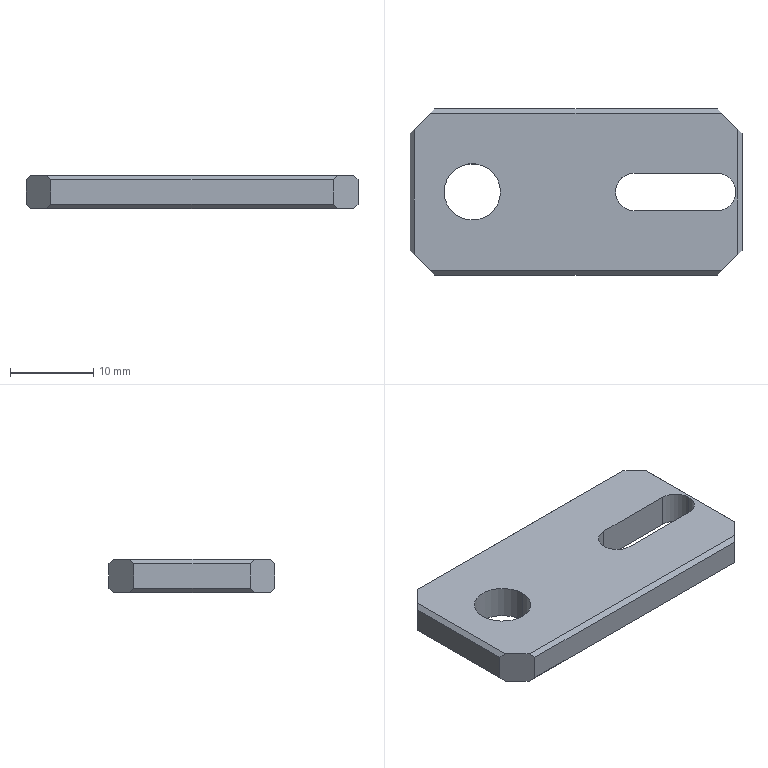Part | SolidWorks | features Chamfer 2, Extrusion 1, HoleWzd 1, ICE 1 | 1 solid | 25 faces | box 40 x 20 x 4 mm | volume 2715 mm3 | plane 20 | cylinder 5 | commonest cylinder face diameters 4.5 x3 6.8 x2
STEP:
#1=CARTESIAN_POINT('',(19.25,0.,0.));
#2=VERTEX_POINT('',#1);
#3=CARTESIAN_POINT('',(17.,2.25,0.));
#4=VERTEX_POINT('',#3);
#5=CARTESIAN_POINT('',(17.,0.,0.));
#6=DIRECTION('',(0.,0.,1.));
#7=DIRECTION('',(1.,0.,0.));
#8=AXIS2_PLACEMENT_3D('',#5,#6,#7);
#9=CIRCLE('',#8,2.25);
#10=EDGE_CURVE('',#2,#4,#9,.T.);
#11=ORIENTED_EDGE('',*,*,#10,.F.);
#12=CARTESIAN_POINT('',(19.25,0.,4.));
#13=VERTEX_POINT('',#12);
#14=CARTESIAN_POINT('',(19.25,0.,0.));
#15=DIRECTION('',(0.,0.,1.));
#16=VECTOR('',#15,1000.);
#17=LINE('',#14,#16);
#18=EDGE_CURVE('',#2,#13,#17,.T.);
#19=ORIENTED_EDGE('',*,*,#18,.T.);
#20=CARTESIAN_POINT('',(17.,2.25,4.));
#21=VERTEX_POINT('',#20);
#22=CARTESIAN_POINT('',(17.,0.,4.));
#23=DIRECTION('',(0.,0.,1.));
#24=DIRECTION('',(1.,0.,0.));
#25=AXIS2_PLACEMENT_3D('',#22,#23,#24);
#26=CIRCLE('',#25,2.25);
#27=EDGE_CURVE('',#13,#21,#26,.T.);
#28=ORIENTED_EDGE('',*,*,#27,.T.);
#29=CARTESIAN_POINT('',(17.,2.25,0.));
#30=DIRECTION('',(0.,0.,1.));
#31=VECTOR('',#30,1000.);
#32=LINE('',#29,#31);
#33=EDGE_CURVE('',#4,#21,#32,.T.);
#34=ORIENTED_EDGE('',*,*,#33,.F.);
#35=EDGE_LOOP('',(#11,#19,#28,#34));
#36=FACE_OUTER_BOUND('',#35,.T.);
#37=CARTESIAN_POINT('',(17.,0.,0.));
#38=DIRECTION('',(0.,0.,1.));
#39=DIRECTION('',(1.,0.,0.));
#40=AXIS2_PLACEMENT_3D('',#37,#38,#39);
#41=CYLINDRICAL_SURFACE('',#40,2.25);
#42=ADVANCED_FACE('',(#36),#41,.F.);
#43=CARTESIAN_POINT('',(-15.9,0.,0.));
#44=VERTEX_POINT('',#43);
#45=CARTESIAN_POINT('',(-9.1,0.,0.));
#46=VERTEX_POINT('',#45);
#47=CARTESIAN_POINT('',(-12.5,0.,0.));
#48=DIRECTION('',(0.,0.,1.));
#49=DIRECTION('',(1.,0.,0.));
#50=AXIS2_PLACEMENT_3D('',#47,#48,#49);
#51=CIRCLE('',#50,3.4);
#52=EDGE_CURVE('',#44,#46,#51,.T.);
#53=ORIENTED_EDGE('',*,*,#52,.F.);
#54=CARTESIAN_POINT('',(-15.9,0.,4.));
#55=VERTEX_POINT('',#54);
#56=CARTESIAN_POINT('',(-15.9,0.,4.));
#57=DIRECTION('',(0.,0.,1.));
#58=VECTOR('',#57,1000.);
#59=LINE('',#56,#58);
#60=EDGE_CURVE('',#44,#55,#59,.T.);
#61=ORIENTED_EDGE('',*,*,#60,.T.);
#62=CARTESIAN_POINT('',(-9.1,0.,4.));
#63=VERTEX_POINT('',#62);
#64=CARTESIAN_POINT('',(-12.5,0.,4.));
#65=DIRECTION('',(0.,0.,1.));
#66=DIRECTION('',(1.,0.,0.));
#67=AXIS2_PLACEMENT_3D('',#64,#65,#66);
#68=CIRCLE('',#67,3.4);
#69=EDGE_CURVE('',#55,#63,#68,.T.);
#70=ORIENTED_EDGE('',*,*,#69,.T.);
#71=CARTESIAN_POINT('',(-9.1,0.,4.));
#72=DIRECTION('',(0.,0.,1.));
#73=VECTOR('',#72,1000.);
#74=LINE('',#71,#73);
#75=EDGE_CURVE('',#46,#63,#74,.T.);
#76=ORIENTED_EDGE('',*,*,#75,.F.);
#77=EDGE_LOOP('',(#53,#61,#70,#76));
#78=FACE_OUTER_BOUND('',#77,.T.);
#79=CARTESIAN_POINT('',(-12.5,0.,4.));
#80=DIRECTION('',(0.,0.,1.));
#81=DIRECTION('',(1.,0.,0.));
#82=AXIS2_PLACEMENT_3D('',#79,#80,#81);
#83=CYLINDRICAL_SURFACE('',#82,3.4);
#84=ADVANCED_FACE('',(#78),#83,.F.);
#85=CARTESIAN_POINT('',(20.,-7.,3.5));
#86=VERTEX_POINT('',#85);
#87=CARTESIAN_POINT('',(20.,-7.,0.5));
#88=VERTEX_POINT('',#87);
#89=CARTESIAN_POINT('',(20.,-7.,4.));
#90=DIRECTION('',(0.,0.,-1.));
#91=VECTOR('',#90,1000.);
#92=LINE('',#89,#91);
#93=EDGE_CURVE('',#86,#88,#92,.T.);
#94=ORIENTED_EDGE('',*,*,#93,.T.);
#95=CARTESIAN_POINT('',(20.,7.,0.5));
#96=VERTEX_POINT('',#95);
#97=CARTESIAN_POINT('',(20.,7.,0.5));
#98=DIRECTION('',(0.,1.,0.));
#99=VECTOR('',#98,1000.);
#100=LINE('',#97,#99);
#101=EDGE_CURVE('',#88,#96,#100,.T.);
#102=ORIENTED_EDGE('',*,*,#101,.T.);
#103=CARTESIAN_POINT('',(20.,7.,3.5));
#104=VERTEX_POINT('',#103);
#105=CARTESIAN_POINT('',(20.,7.,4.));
#106=DIRECTION('',(0.,0.,1.));
#107=VECTOR('',#106,1000.);
#108=LINE('',#105,#107);
#109=EDGE_CURVE('',#96,#104,#108,.T.);
#110=ORIENTED_EDGE('',*,*,#109,.T.);
#111=CARTESIAN_POINT('',(20.,-10.,3.5));
#112=DIRECTION('',(0.,-1.,0.));
#113=VECTOR('',#112,1000.);
#114=LINE('',#111,#113);
#115=EDGE_CURVE('',#104,#86,#114,.T.);
#116=ORIENTED_EDGE('',*,*,#115,.T.);
#117=EDGE_LOOP('',(#94,#102,#110,#116));
#118=FACE_OUTER_BOUND('',#117,.T.);
#119=CARTESIAN_POINT('',(20.,-10.,4.));
#120=DIRECTION('',(-1.,0.,0.));
#121=DIRECTION('',(0.,0.,1.));
#122=AXIS2_PLACEMENT_3D('',#119,#120,#121);
#123=PLANE('',#122);
#124=ADVANCED_FACE('',(#118),#123,.F.);
#125=CARTESIAN_POINT('',(17.,10.,3.5));
#126=VERTEX_POINT('',#125);
#127=CARTESIAN_POINT('',(17.,10.,0.5));
#128=VERTEX_POINT('',#127);
#129=CARTESIAN_POINT('',(17.,10.,4.));
#130=DIRECTION('',(0.,0.,-1.));
#131=VECTOR('',#130,1000.);
#132=LINE('',#129,#131);
#133=EDGE_CURVE('',#126,#128,#132,.T.);
#134=ORIENTED_EDGE('',*,*,#133,.T.);
#135=CARTESIAN_POINT('',(-17.,10.,0.5));
#136=VERTEX_POINT('',#135);
#137=CARTESIAN_POINT('',(-17.,10.,0.5));
#138=DIRECTION('',(-1.,0.,0.));
#139=VECTOR('',#138,1000.);
#140=LINE('',#137,#139);
#141=EDGE_CURVE('',#128,#136,#140,.T.);
#142=ORIENTED_EDGE('',*,*,#141,.T.);
#143=CARTESIAN_POINT('',(-17.,10.,3.5));
#144=VERTEX_POINT('',#143);
#145=CARTESIAN_POINT('',(-17.,10.,4.));
#146=DIRECTION('',(0.,0.,1.));
#147=VECTOR('',#146,1000.);
#148=LINE('',#145,#147);
#149=EDGE_CURVE('',#136,#144,#148,.T.);
#150=ORIENTED_EDGE('',*,*,#149,.T.);
#151=CARTESIAN_POINT('',(-20.,10.,3.5));
#152=DIRECTION('',(1.,0.,0.));
#153=VECTOR('',#152,1000.);
#154=LINE('',#151,#153);
#155=EDGE_CURVE('',#144,#126,#154,.T.);
#156=ORIENTED_EDGE('',*,*,#155,.T.);
#157=EDGE_LOOP('',(#134,#142,#150,#156));
#158=FACE_OUTER_BOUND('',#157,.T.);
#159=CARTESIAN_POINT('',(-20.,10.,4.));
#160=DIRECTION('',(0.,-1.,0.));
#161=DIRECTION('',(0.,0.,-1.));
#162=AXIS2_PLACEMENT_3D('',#159,#160,#161);
#163=PLANE('',#162);
#164=ADVANCED_FACE('',(#158),#163,.F.);
#165=CARTESIAN_POINT('',(-20.,-7.,0.5));
#166=VERTEX_POINT('',#165);
#167=CARTESIAN_POINT('',(-20.,-7.,3.5));
#168=VERTEX_POINT('',#167);
#169=CARTESIAN_POINT('',(-20.,-7.,4.));
#170=DIRECTION('',(0.,0.,1.));
#171=VECTOR('',#170,1000.);
#172=LINE('',#169,#171);
#173=EDGE_CURVE('',#166,#168,#172,.T.);
#174=ORIENTED_EDGE('',*,*,#173,.T.);
#175=CARTESIAN_POINT('',(-20.,7.,3.5));
#176=VERTEX_POINT('',#175);
#177=CARTESIAN_POINT('',(-20.,-10.,3.5));
#178=DIRECTION('',(0.,1.,0.));
#179=VECTOR('',#178,1000.);
#180=LINE('',#177,#179);
#181=EDGE_CURVE('',#168,#176,#180,.T.);
#182=ORIENTED_EDGE('',*,*,#181,.T.);
#183=CARTESIAN_POINT('',(-20.,7.,0.5));
#184=VERTEX_POINT('',#183);
#185=CARTESIAN_POINT('',(-20.,7.,4.));
#186=DIRECTION('',(0.,0.,-1.));
#187=VECTOR('',#186,1000.);
#188=LINE('',#185,#187);
#189=EDGE_CURVE('',#176,#184,#188,.T.);
#190=ORIENTED_EDGE('',*,*,#189,.T.);
#191=CARTESIAN_POINT('',(-20.,-7.,0.5));
#192=DIRECTION('',(0.,-1.,0.));
#193=VECTOR('',#192,1000.);
#194=LINE('',#191,#193);
#195=EDGE_CURVE('',#184,#166,#194,.T.);
#196=ORIENTED_EDGE('',*,*,#195,.T.);
#197=EDGE_LOOP('',(#174,#182,#190,#196));
#198=FACE_OUTER_BOUND('',#197,.T.);
#199=CARTESIAN_POINT('',(-20.,-10.,4.));
#200=DIRECTION('',(1.,0.,0.));
#201=DIRECTION('',(0.,0.,-1.));
#202=AXIS2_PLACEMENT_3D('',#199,#200,#201);
#203=PLANE('',#202);
#204=ADVANCED_FACE('',(#198),#203,.F.);
#205=CARTESIAN_POINT('',(-17.,-10.,3.5));
#206=VERTEX_POINT('',#205);
#207=CARTESIAN_POINT('',(-17.,-10.,0.5));
#208=VERTEX_POINT('',#207);
#209=CARTESIAN_POINT('',(-17.,-10.,4.));
#210=DIRECTION('',(0.,0.,-1.));
#211=VECTOR('',#210,1000.);
#212=LINE('',#209,#211);
#213=EDGE_CURVE('',#206,#208,#212,.T.);
#214=ORIENTED_EDGE('',*,*,#213,.T.);
#215=CARTESIAN_POINT('',(17.,-10.,0.5));
#216=VERTEX_POINT('',#215);
#217=CARTESIAN_POINT('',(17.,-10.,0.5));
#218=DIRECTION('',(1.,0.,0.));
#219=VECTOR('',#218,1000.);
#220=LINE('',#217,#219);
#221=EDGE_CURVE('',#208,#216,#220,.T.);
#222=ORIENTED_EDGE('',*,*,#221,.T.);
#223=CARTESIAN_POINT('',(17.,-10.,3.5));
#224=VERTEX_POINT('',#223);
#225=CARTESIAN_POINT('',(17.,-10.,4.));
#226=DIRECTION('',(0.,0.,1.));
#227=VECTOR('',#226,1000.);
#228=LINE('',#225,#227);
#229=EDGE_CURVE('',#216,#224,#228,.T.);
#230=ORIENTED_EDGE('',*,*,#229,.T.);
#231=CARTESIAN_POINT('',(-20.,-10.,3.5));
#232=DIRECTION('',(-1.,0.,0.));
#233=VECTOR('',#232,1000.);
#234=LINE('',#231,#233);
#235=EDGE_CURVE('',#224,#206,#234,.T.);
#236=ORIENTED_EDGE('',*,*,#235,.T.);
#237=EDGE_LOOP('',(#214,#222,#230,#236));
#238=FACE_OUTER_BOUND('',#237,.T.);
#239=CARTESIAN_POINT('',(-20.,-10.,4.));
#240=DIRECTION('',(0.,1.,0.));
#241=DIRECTION('',(0.,0.,1.));
#242=AXIS2_PLACEMENT_3D('',#239,#240,#241);
#243=PLANE('',#242);
#244=ADVANCED_FACE('',(#238),#243,.F.);
#245=CARTESIAN_POINT('',(7.,-2.25,4.));
#246=VERTEX_POINT('',#245);
#247=CARTESIAN_POINT('',(17.,-2.25,4.));
#248=VERTEX_POINT('',#247);
#249=CARTESIAN_POINT('',(7.,-2.25,4.));
#250=DIRECTION('',(1.,0.,0.));
#251=VECTOR('',#250,1000.);
#252=LINE('',#249,#251);
#253=EDGE_CURVE('',#246,#248,#252,.T.);
#254=ORIENTED_EDGE('',*,*,#253,.F.);
#255=CARTESIAN_POINT('',(7.,2.25,4.));
#256=VERTEX_POINT('',#255);
#257=CARTESIAN_POINT('',(7.,0.,4.));
#258=DIRECTION('',(0.,0.,1.));
#259=DIRECTION('',(1.,0.,0.));
#260=AXIS2_PLACEMENT_3D('',#257,#258,#259);
#261=CIRCLE('',#260,2.25);
#262=EDGE_CURVE('',#256,#246,#261,.T.);
#263=ORIENTED_EDGE('',*,*,#262,.F.);
#264=CARTESIAN_POINT('',(7.,2.25,4.));
#265=DIRECTION('',(-1.,0.,0.));
#266=VECTOR('',#265,1000.);
#267=LINE('',#264,#266);
#268=EDGE_CURVE('',#21,#256,#267,.T.);
#269=ORIENTED_EDGE('',*,*,#268,.F.);
#270=ORIENTED_EDGE('',*,*,#27,.F.);
#271=CARTESIAN_POINT('',(17.,0.,4.));
#272=DIRECTION('',(0.,0.,1.));
#273=DIRECTION('',(1.,0.,0.));
#274=AXIS2_PLACEMENT_3D('',#271,#272,#273);
#275=CIRCLE('',#274,2.25);
#276=EDGE_CURVE('',#248,#13,#275,.T.);
#277=ORIENTED_EDGE('',*,*,#276,.F.);
#278=EDGE_LOOP('',(#254,#263,#269,#270,#277));
#279=FACE_BOUND('',#278,.T.);
#280=CARTESIAN_POINT('',(-12.5,0.,4.));
#281=DIRECTION('',(0.,0.,1.));
#282=DIRECTION('',(1.,0.,0.));
#283=AXIS2_PLACEMENT_3D('',#280,#281,#282);
#284=CIRCLE('',#283,3.4);
#285=EDGE_CURVE('',#63,#55,#284,.T.);
#286=ORIENTED_EDGE('',*,*,#285,.F.);
#287=ORIENTED_EDGE('',*,*,#69,.F.);
#288=EDGE_LOOP('',(#286,#287));
#289=FACE_BOUND('',#288,.T.);
#290=CARTESIAN_POINT('',(17.5,-9.5,4.));
#291=VERTEX_POINT('',#290);
#292=CARTESIAN_POINT('',(19.5,-7.5,4.));
#293=VERTEX_POINT('',#292);
#294=CARTESIAN_POINT('',(20.,-7.,4.));
#295=DIRECTION('',(0.7071,0.7071,0.));
#296=VECTOR('',#295,1000.);
#297=LINE('',#294,#296);
#298=EDGE_CURVE('',#291,#293,#297,.T.);
#299=ORIENTED_EDGE('',*,*,#298,.T.);
#300=CARTESIAN_POINT('',(19.5,7.5,4.));
#301=VERTEX_POINT('',#300);
#302=CARTESIAN_POINT('',(19.5,0.,4.));
#303=DIRECTION('',(0.,1.,0.));
#304=VECTOR('',#303,1000.);
#305=LINE('',#302,#304);
#306=EDGE_CURVE('',#293,#301,#305,.T.);
#307=ORIENTED_EDGE('',*,*,#306,.T.);
#308=CARTESIAN_POINT('',(17.5,9.5,4.));
#309=VERTEX_POINT('',#308);
#310=CARTESIAN_POINT('',(17.,10.,4.));
#311=DIRECTION('',(-0.7071,0.7071,0.));
#312=VECTOR('',#311,1000.);
#313=LINE('',#310,#312);
#314=EDGE_CURVE('',#301,#309,#313,.T.);
#315=ORIENTED_EDGE('',*,*,#314,.T.);
#316=CARTESIAN_POINT('',(-17.5,9.5,4.));
#317=VERTEX_POINT('',#316);
#318=CARTESIAN_POINT('',(0.,9.5,4.));
#319=DIRECTION('',(-1.,0.,0.));
#320=VECTOR('',#319,1000.);
#321=LINE('',#318,#320);
#322=EDGE_CURVE('',#309,#317,#321,.T.);
#323=ORIENTED_EDGE('',*,*,#322,.T.);
#324=CARTESIAN_POINT('',(-19.5,7.5,4.));
#325=VERTEX_POINT('',#324);
#326=CARTESIAN_POINT('',(-20.,7.,4.));
#327=DIRECTION('',(-0.7071,-0.7071,0.));
#328=VECTOR('',#327,1000.);
#329=LINE('',#326,#328);
#330=EDGE_CURVE('',#317,#325,#329,.T.);
#331=ORIENTED_EDGE('',*,*,#330,.T.);
#332=CARTESIAN_POINT('',(-19.5,-7.5,4.));
#333=VERTEX_POINT('',#332);
#334=CARTESIAN_POINT('',(-19.5,0.,4.));
#335=DIRECTION('',(0.,-1.,0.));
#336=VECTOR('',#335,1000.);
#337=LINE('',#334,#336);
#338=EDGE_CURVE('',#325,#333,#337,.T.);
#339=ORIENTED_EDGE('',*,*,#338,.T.);
#340=CARTESIAN_POINT('',(-17.5,-9.5,4.));
#341=VERTEX_POINT('',#340);
#342=CARTESIAN_POINT('',(-17.,-10.,4.));
#343=DIRECTION('',(0.7071,-0.7071,0.));
#344=VECTOR('',#343,1000.);
#345=LINE('',#342,#344);
#346=EDGE_CURVE('',#333,#341,#345,.T.);
#347=ORIENTED_EDGE('',*,*,#346,.T.);
#348=CARTESIAN_POINT('',(0.,-9.5,4.));
#349=DIRECTION('',(1.,0.,0.));
#350=VECTOR('',#349,1000.);
#351=LINE('',#348,#350);
#352=EDGE_CURVE('',#341,#291,#351,.T.);
#353=ORIENTED_EDGE('',*,*,#352,.T.);
#354=EDGE_LOOP('',(#299,#307,#315,#323,#331,#339,#347,#353));
#355=FACE_OUTER_BOUND('',#354,.T.);
#356=CARTESIAN_POINT('',(0.,0.,4.));
#357=DIRECTION('',(0.,0.,-1.));
#358=DIRECTION('',(-1.,0.,0.));
#359=AXIS2_PLACEMENT_3D('',#356,#357,#358);
#360=PLANE('',#359);
#361=ADVANCED_FACE('',(#279,#289,#355),#360,.F.);
#362=CARTESIAN_POINT('',(7.,2.25,0.));
#363=VERTEX_POINT('',#362);
#364=CARTESIAN_POINT('',(7.,-2.25,0.));
#365=VERTEX_POINT('',#364);
#366=CARTESIAN_POINT('',(7.,0.,0.));
#367=DIRECTION('',(0.,0.,1.));
#368=DIRECTION('',(1.,0.,0.));
#369=AXIS2_PLACEMENT_3D('',#366,#367,#368);
#370=CIRCLE('',#369,2.25);
#371=EDGE_CURVE('',#363,#365,#370,.T.);
#372=ORIENTED_EDGE('',*,*,#371,.T.);
#373=CARTESIAN_POINT('',(17.,-2.25,0.));
#374=VERTEX_POINT('',#373);
#375=CARTESIAN_POINT('',(7.,-2.25,0.));
#376=DIRECTION('',(1.,0.,0.));
#377=VECTOR('',#376,1000.);
#378=LINE('',#375,#377);
#379=EDGE_CURVE('',#365,#374,#378,.T.);
#380=ORIENTED_EDGE('',*,*,#379,.T.);
#381=CARTESIAN_POINT('',(17.,0.,0.));
#382=DIRECTION('',(0.,0.,1.));
#383=DIRECTION('',(1.,0.,0.));
#384=AXIS2_PLACEMENT_3D('',#381,#382,#383);
#385=CIRCLE('',#384,2.25);
#386=EDGE_CURVE('',#374,#2,#385,.T.);
#387=ORIENTED_EDGE('',*,*,#386,.T.);
#388=ORIENTED_EDGE('',*,*,#10,.T.);
#389=CARTESIAN_POINT('',(7.,2.25,0.));
#390=DIRECTION('',(-1.,0.,0.));
#391=VECTOR('',#390,1000.);
#392=LINE('',#389,#391);
#393=EDGE_CURVE('',#4,#363,#392,.T.);
#394=ORIENTED_EDGE('',*,*,#393,.T.);
#395=EDGE_LOOP('',(#372,#380,#387,#388,#394));
#396=FACE_BOUND('',#395,.T.);
#397=CARTESIAN_POINT('',(-12.5,0.,0.));
#398=DIRECTION('',(0.,0.,1.));
#399=DIRECTION('',(1.,0.,0.));
#400=AXIS2_PLACEMENT_3D('',#397,#398,#399);
#401=CIRCLE('',#400,3.4);
#402=EDGE_CURVE('',#46,#44,#401,.T.);
#403=ORIENTED_EDGE('',*,*,#402,.T.);
#404=ORIENTED_EDGE('',*,*,#52,.T.);
#405=EDGE_LOOP('',(#403,#404));
#406=FACE_BOUND('',#405,.T.);
#407=CARTESIAN_POINT('',(17.5,9.5,0.));
#408=VERTEX_POINT('',#407);
#409=CARTESIAN_POINT('',(19.5,7.5,0.));
#410=VERTEX_POINT('',#409);
#411=CARTESIAN_POINT('',(13.5,13.5,0.));
#412=DIRECTION('',(0.7071,-0.7071,0.));
#413=VECTOR('',#412,1000.);
#414=LINE('',#411,#413);
#415=EDGE_CURVE('',#408,#410,#414,.T.);
#416=ORIENTED_EDGE('',*,*,#415,.T.);
#417=CARTESIAN_POINT('',(19.5,-7.5,0.));
#418=VERTEX_POINT('',#417);
#419=CARTESIAN_POINT('',(19.5,-7.,0.));
#420=DIRECTION('',(0.,-1.,0.));
#421=VECTOR('',#420,1000.);
#422=LINE('',#419,#421);
#423=EDGE_CURVE('',#410,#418,#422,.T.);
#424=ORIENTED_EDGE('',*,*,#423,.T.);
#425=CARTESIAN_POINT('',(17.5,-9.5,0.));
#426=VERTEX_POINT('',#425);
#427=CARTESIAN_POINT('',(13.5,-13.5,0.));
#428=DIRECTION('',(-0.7071,-0.7071,0.));
#429=VECTOR('',#428,1000.);
#430=LINE('',#427,#429);
#431=EDGE_CURVE('',#418,#426,#430,.T.);
#432=ORIENTED_EDGE('',*,*,#431,.T.);
#433=CARTESIAN_POINT('',(-17.5,-9.5,0.));
#434=VERTEX_POINT('',#433);
#435=CARTESIAN_POINT('',(-17.,-9.5,0.));
#436=DIRECTION('',(-1.,0.,0.));
#437=VECTOR('',#436,1000.);
#438=LINE('',#435,#437);
#439=EDGE_CURVE('',#426,#434,#438,.T.);
#440=ORIENTED_EDGE('',*,*,#439,.T.);
#441=CARTESIAN_POINT('',(-19.5,-7.5,0.));
#442=VERTEX_POINT('',#441);
#443=CARTESIAN_POINT('',(-13.5,-13.5,0.));
#444=DIRECTION('',(-0.7071,0.7071,0.));
#445=VECTOR('',#444,1000.);
#446=LINE('',#443,#445);
#447=EDGE_CURVE('',#434,#442,#446,.T.);
#448=ORIENTED_EDGE('',*,*,#447,.T.);
#449=CARTESIAN_POINT('',(-19.5,7.5,0.));
#450=VERTEX_POINT('',#449);
#451=CARTESIAN_POINT('',(-19.5,7.,0.));
#452=DIRECTION('',(0.,1.,0.));
#453=VECTOR('',#452,1000.);
#454=LINE('',#451,#453);
#455=EDGE_CURVE('',#442,#450,#454,.T.);
#456=ORIENTED_EDGE('',*,*,#455,.T.);
#457=CARTESIAN_POINT('',(-17.5,9.5,0.));
#458=VERTEX_POINT('',#457);
#459=CARTESIAN_POINT('',(-13.5,13.5,0.));
#460=DIRECTION('',(0.7071,0.7071,0.));
#461=VECTOR('',#460,1000.);
#462=LINE('',#459,#461);
#463=EDGE_CURVE('',#450,#458,#462,.T.);
#464=ORIENTED_EDGE('',*,*,#463,.T.);
#465=CARTESIAN_POINT('',(17.,9.5,0.));
#466=DIRECTION('',(1.,0.,0.));
#467=VECTOR('',#466,1000.);
#468=LINE('',#465,#467);
#469=EDGE_CURVE('',#458,#408,#468,.T.);
#470=ORIENTED_EDGE('',*,*,#469,.T.);
#471=EDGE_LOOP('',(#416,#424,#432,#440,#448,#456,#464,#470));
#472=FACE_OUTER_BOUND('',#471,.T.);
#473=CARTESIAN_POINT('',(0.,0.,0.));
#474=DIRECTION('',(0.,0.,-1.));
#475=DIRECTION('',(-1.,0.,0.));
#476=AXIS2_PLACEMENT_3D('',#473,#474,#475);
#477=PLANE('',#476);
#478=ADVANCED_FACE('',(#396,#406,#472),#477,.T.);
#479=ORIENTED_EDGE('',*,*,#60,.F.);
#480=ORIENTED_EDGE('',*,*,#402,.F.);
#481=ORIENTED_EDGE('',*,*,#75,.T.);
#482=ORIENTED_EDGE('',*,*,#285,.T.);
#483=EDGE_LOOP('',(#479,#480,#481,#482));
#484=FACE_OUTER_BOUND('',#483,.T.);
#485=CARTESIAN_POINT('',(-12.5,0.,4.));
#486=DIRECTION('',(0.,0.,1.));
#487=DIRECTION('',(1.,0.,0.));
#488=AXIS2_PLACEMENT_3D('',#485,#486,#487);
#489=CYLINDRICAL_SURFACE('',#488,3.4);
#490=ADVANCED_FACE('',(#484),#489,.F.);
#491=ORIENTED_EDGE('',*,*,#262,.T.);
#492=CARTESIAN_POINT('',(7.,-2.25,0.));
#493=DIRECTION('',(0.,0.,1.));
#494=VECTOR('',#493,1000.);
#495=LINE('',#492,#494);
#496=EDGE_CURVE('',#365,#246,#495,.T.);
#497=ORIENTED_EDGE('',*,*,#496,.F.);
#498=ORIENTED_EDGE('',*,*,#371,.F.);
#499=CARTESIAN_POINT('',(7.,2.25,0.));
#500=DIRECTION('',(0.,0.,1.));
#501=VECTOR('',#500,1000.);
#502=LINE('',#499,#501);
#503=EDGE_CURVE('',#363,#256,#502,.T.);
#504=ORIENTED_EDGE('',*,*,#503,.T.);
#505=EDGE_LOOP('',(#491,#497,#498,#504));
#506=FACE_OUTER_BOUND('',#505,.T.);
#507=CARTESIAN_POINT('',(7.,0.,0.));
#508=DIRECTION('',(0.,0.,1.));
#509=DIRECTION('',(1.,0.,0.));
#510=AXIS2_PLACEMENT_3D('',#507,#508,#509);
#511=CYLINDRICAL_SURFACE('',#510,2.25);
#512=ADVANCED_FACE('',(#506),#511,.F.);
#513=ORIENTED_EDGE('',*,*,#268,.T.);
#514=ORIENTED_EDGE('',*,*,#503,.F.);
#515=ORIENTED_EDGE('',*,*,#393,.F.);
#516=ORIENTED_EDGE('',*,*,#33,.T.);
#517=EDGE_LOOP('',(#513,#514,#515,#516));
#518=FACE_OUTER_BOUND('',#517,.T.);
#519=CARTESIAN_POINT('',(7.,2.25,0.));
#520=DIRECTION('',(0.,1.,0.));
#521=DIRECTION('',(0.,0.,1.));
#522=AXIS2_PLACEMENT_3D('',#519,#520,#521);
#523=PLANE('',#522);
#524=ADVANCED_FACE('',(#518),#523,.F.);
#525=ORIENTED_EDGE('',*,*,#18,.F.);
#526=ORIENTED_EDGE('',*,*,#386,.F.);
#527=CARTESIAN_POINT('',(17.,-2.25,0.));
#528=DIRECTION('',(0.,0.,1.));
#529=VECTOR('',#528,1000.);
#530=LINE('',#527,#529);
#531=EDGE_CURVE('',#374,#248,#530,.T.);
#532=ORIENTED_EDGE('',*,*,#531,.T.);
#533=ORIENTED_EDGE('',*,*,#276,.T.);
#534=EDGE_LOOP('',(#525,#526,#532,#533));
#535=FACE_OUTER_BOUND('',#534,.T.);
#536=CARTESIAN_POINT('',(17.,0.,0.));
#537=DIRECTION('',(0.,0.,1.));
#538=DIRECTION('',(1.,0.,0.));
#539=AXIS2_PLACEMENT_3D('',#536,#537,#538);
#540=CYLINDRICAL_SURFACE('',#539,2.25);
#541=ADVANCED_FACE('',(#535),#540,.F.);
#542=ORIENTED_EDGE('',*,*,#253,.T.);
#543=ORIENTED_EDGE('',*,*,#531,.F.);
#544=ORIENTED_EDGE('',*,*,#379,.F.);
#545=ORIENTED_EDGE('',*,*,#496,.T.);
#546=EDGE_LOOP('',(#542,#543,#544,#545));
#547=FACE_OUTER_BOUND('',#546,.T.);
#548=CARTESIAN_POINT('',(7.,-2.25,0.));
#549=DIRECTION('',(0.,-1.,0.));
#550=DIRECTION('',(0.,0.,-1.));
#551=AXIS2_PLACEMENT_3D('',#548,#549,#550);
#552=PLANE('',#551);
#553=ADVANCED_FACE('',(#547),#552,.F.);
#554=ORIENTED_EDGE('',*,*,#431,.F.);
#555=CARTESIAN_POINT('',(21.167,-5.833,1.667));
#556=DIRECTION('',(0.5774,0.5774,0.5774));
#557=VECTOR('',#556,1000.);
#558=LINE('',#555,#557);
#559=EDGE_CURVE('',#418,#88,#558,.T.);
#560=ORIENTED_EDGE('',*,*,#559,.T.);
#561=ORIENTED_EDGE('',*,*,#93,.F.);
#562=CARTESIAN_POINT('',(19.833,-7.167,3.667));
#563=DIRECTION('',(-0.5774,-0.5774,0.5774));
#564=VECTOR('',#563,1000.);
#565=LINE('',#562,#564);
#566=EDGE_CURVE('',#86,#293,#565,.T.);
#567=ORIENTED_EDGE('',*,*,#566,.T.);
#568=ORIENTED_EDGE('',*,*,#298,.F.);
#569=CARTESIAN_POINT('',(19.167,-7.833,5.667));
#570=DIRECTION('',(-0.5774,-0.5774,-0.5774));
#571=VECTOR('',#570,1000.);
#572=LINE('',#569,#571);
#573=EDGE_CURVE('',#291,#224,#572,.T.);
#574=ORIENTED_EDGE('',*,*,#573,.T.);
#575=ORIENTED_EDGE('',*,*,#229,.F.);
#576=CARTESIAN_POINT('',(17.833,-9.167,-0.3333));
#577=DIRECTION('',(0.5774,0.5774,-0.5774));
#578=VECTOR('',#577,1000.);
#579=LINE('',#576,#578);
#580=EDGE_CURVE('',#216,#426,#579,.T.);
#581=ORIENTED_EDGE('',*,*,#580,.T.);
#582=EDGE_LOOP('',(#554,#560,#561,#567,#568,#574,#575,#581));
#583=FACE_OUTER_BOUND('',#582,.T.);
#584=CARTESIAN_POINT('',(20.,-7.,4.));
#585=DIRECTION('',(-0.7071,0.7071,0.));
#586=DIRECTION('',(0.,0.,-1.));
#587=AXIS2_PLACEMENT_3D('',#584,#585,#586);
#588=PLANE('',#587);
#589=ADVANCED_FACE('',(#583),#588,.F.);
#590=ORIENTED_EDGE('',*,*,#346,.F.);
#591=CARTESIAN_POINT('',(-17.833,-9.167,5.667));
#592=DIRECTION('',(-0.5774,0.5774,-0.5774));
#593=VECTOR('',#592,1000.);
#594=LINE('',#591,#593);
#595=EDGE_CURVE('',#333,#168,#594,.T.);
#596=ORIENTED_EDGE('',*,*,#595,.T.);
#597=ORIENTED_EDGE('',*,*,#173,.F.);
#598=CARTESIAN_POINT('',(-19.167,-7.833,-0.3333));
#599=DIRECTION('',(0.5774,-0.5774,-0.5774));
#600=VECTOR('',#599,1000.);
#601=LINE('',#598,#600);
#602=EDGE_CURVE('',#166,#442,#601,.T.);
#603=ORIENTED_EDGE('',*,*,#602,.T.);
#604=ORIENTED_EDGE('',*,*,#447,.F.);
#605=CARTESIAN_POINT('',(-15.833,-11.167,1.667));
#606=DIRECTION('',(0.5774,-0.5774,0.5774));
#607=VECTOR('',#606,1000.);
#608=LINE('',#605,#607);
#609=EDGE_CURVE('',#434,#208,#608,.T.);
#610=ORIENTED_EDGE('',*,*,#609,.T.);
#611=ORIENTED_EDGE('',*,*,#213,.F.);
#612=CARTESIAN_POINT('',(-17.167,-9.833,3.667));
#613=DIRECTION('',(-0.5774,0.5774,0.5774));
#614=VECTOR('',#613,1000.);
#615=LINE('',#612,#614);
#616=EDGE_CURVE('',#206,#341,#615,.T.);
#617=ORIENTED_EDGE('',*,*,#616,.T.);
#618=EDGE_LOOP('',(#590,#596,#597,#603,#604,#610,#611,#617));
#619=FACE_OUTER_BOUND('',#618,.T.);
#620=CARTESIAN_POINT('',(-17.,-10.,4.));
#621=DIRECTION('',(0.7071,0.7071,0.));
#622=DIRECTION('',(0.,0.,-1.));
#623=AXIS2_PLACEMENT_3D('',#620,#621,#622);
#624=PLANE('',#623);
#625=ADVANCED_FACE('',(#619),#624,.F.);
#626=ORIENTED_EDGE('',*,*,#189,.F.);
#627=CARTESIAN_POINT('',(-19.833,7.167,3.667));
#628=DIRECTION('',(0.5774,0.5774,0.5774));
#629=VECTOR('',#628,1000.);
#630=LINE('',#627,#629);
#631=EDGE_CURVE('',#176,#325,#630,.T.);
#632=ORIENTED_EDGE('',*,*,#631,.T.);
#633=ORIENTED_EDGE('',*,*,#330,.F.);
#634=CARTESIAN_POINT('',(-19.167,7.833,5.667));
#635=DIRECTION('',(0.5774,0.5774,-0.5774));
#636=VECTOR('',#635,1000.);
#637=LINE('',#634,#636);
#638=EDGE_CURVE('',#317,#144,#637,.T.);
#639=ORIENTED_EDGE('',*,*,#638,.T.);
#640=ORIENTED_EDGE('',*,*,#149,.F.);
#641=CARTESIAN_POINT('',(-17.833,9.167,-0.3333));
#642=DIRECTION('',(-0.5774,-0.5774,-0.5774));
#643=VECTOR('',#642,1000.);
#644=LINE('',#641,#643);
#645=EDGE_CURVE('',#136,#458,#644,.T.);
#646=ORIENTED_EDGE('',*,*,#645,.T.);
#647=ORIENTED_EDGE('',*,*,#463,.F.);
#648=CARTESIAN_POINT('',(-21.167,5.833,1.667));
#649=DIRECTION('',(-0.5774,-0.5774,0.5774));
#650=VECTOR('',#649,1000.);
#651=LINE('',#648,#650);
#652=EDGE_CURVE('',#450,#184,#651,.T.);
#653=ORIENTED_EDGE('',*,*,#652,.T.);
#654=EDGE_LOOP('',(#626,#632,#633,#639,#640,#646,#647,#653));
#655=FACE_OUTER_BOUND('',#654,.T.);
#656=CARTESIAN_POINT('',(-20.,7.,4.));
#657=DIRECTION('',(0.7071,-0.7071,0.));
#658=DIRECTION('',(0.,0.,-1.));
#659=AXIS2_PLACEMENT_3D('',#656,#657,#658);
#660=PLANE('',#659);
#661=ADVANCED_FACE('',(#655),#660,.F.);
#662=ORIENTED_EDGE('',*,*,#109,.F.);
#663=CARTESIAN_POINT('',(19.167,7.833,-0.3333));
#664=DIRECTION('',(-0.5774,0.5774,-0.5774));
#665=VECTOR('',#664,1000.);
#666=LINE('',#663,#665);
#667=EDGE_CURVE('',#96,#410,#666,.T.);
#668=ORIENTED_EDGE('',*,*,#667,.T.);
#669=ORIENTED_EDGE('',*,*,#415,.F.);
#670=CARTESIAN_POINT('',(15.833,11.167,1.667));
#671=DIRECTION('',(-0.5774,0.5774,0.5774));
#672=VECTOR('',#671,1000.);
#673=LINE('',#670,#672);
#674=EDGE_CURVE('',#408,#128,#673,.T.);
#675=ORIENTED_EDGE('',*,*,#674,.T.);
#676=ORIENTED_EDGE('',*,*,#133,.F.);
#677=CARTESIAN_POINT('',(17.167,9.833,3.667));
#678=DIRECTION('',(0.5774,-0.5774,0.5774));
#679=VECTOR('',#678,1000.);
#680=LINE('',#677,#679);
#681=EDGE_CURVE('',#126,#309,#680,.T.);
#682=ORIENTED_EDGE('',*,*,#681,.T.);
#683=ORIENTED_EDGE('',*,*,#314,.F.);
#684=CARTESIAN_POINT('',(17.833,9.167,5.667));
#685=DIRECTION('',(0.5774,-0.5774,-0.5774));
#686=VECTOR('',#685,1000.);
#687=LINE('',#684,#686);
#688=EDGE_CURVE('',#301,#104,#687,.T.);
#689=ORIENTED_EDGE('',*,*,#688,.T.);
#690=EDGE_LOOP('',(#662,#668,#669,#675,#676,#682,#683,#689));
#691=FACE_OUTER_BOUND('',#690,.T.);
#692=CARTESIAN_POINT('',(17.,10.,4.));
#693=DIRECTION('',(-0.7071,-0.7071,0.));
#694=DIRECTION('',(0.,0.,-1.));
#695=AXIS2_PLACEMENT_3D('',#692,#693,#694);
#696=PLANE('',#695);
#697=ADVANCED_FACE('',(#691),#696,.F.);
#698=ORIENTED_EDGE('',*,*,#559,.F.);
#699=ORIENTED_EDGE('',*,*,#423,.F.);
#700=ORIENTED_EDGE('',*,*,#667,.F.);
#701=ORIENTED_EDGE('',*,*,#101,.F.);
#702=EDGE_LOOP('',(#698,#699,#700,#701));
#703=FACE_OUTER_BOUND('',#702,.T.);
#704=CARTESIAN_POINT('',(20.,-10.,0.5));
#705=DIRECTION('',(0.7071,0.,-0.7071));
#706=DIRECTION('',(0.,-1.,0.));
#707=AXIS2_PLACEMENT_3D('',#704,#705,#706);
#708=PLANE('',#707);
#709=ADVANCED_FACE('',(#703),#708,.T.);
#710=ORIENTED_EDGE('',*,*,#566,.F.);
#711=ORIENTED_EDGE('',*,*,#115,.F.);
#712=ORIENTED_EDGE('',*,*,#688,.F.);
#713=ORIENTED_EDGE('',*,*,#306,.F.);
#714=EDGE_LOOP('',(#710,#711,#712,#713));
#715=FACE_OUTER_BOUND('',#714,.T.);
#716=CARTESIAN_POINT('',(19.5,0.,4.));
#717=DIRECTION('',(-0.7071,0.,-0.7071));
#718=DIRECTION('',(0.,1.,0.));
#719=AXIS2_PLACEMENT_3D('',#716,#717,#718);
#720=PLANE('',#719);
#721=ADVANCED_FACE('',(#715),#720,.F.);
#722=ORIENTED_EDGE('',*,*,#631,.F.);
#723=ORIENTED_EDGE('',*,*,#181,.F.);
#724=ORIENTED_EDGE('',*,*,#595,.F.);
#725=ORIENTED_EDGE('',*,*,#338,.F.);
#726=EDGE_LOOP('',(#722,#723,#724,#725));
#727=FACE_OUTER_BOUND('',#726,.T.);
#728=CARTESIAN_POINT('',(-19.5,0.,4.));
#729=DIRECTION('',(0.7071,0.,-0.7071));
#730=DIRECTION('',(0.,-1.,0.));
#731=AXIS2_PLACEMENT_3D('',#728,#729,#730);
#732=PLANE('',#731);
#733=ADVANCED_FACE('',(#727),#732,.F.);
#734=ORIENTED_EDGE('',*,*,#652,.F.);
#735=ORIENTED_EDGE('',*,*,#455,.F.);
#736=ORIENTED_EDGE('',*,*,#602,.F.);
#737=ORIENTED_EDGE('',*,*,#195,.F.);
#738=EDGE_LOOP('',(#734,#735,#736,#737));
#739=FACE_OUTER_BOUND('',#738,.T.);
#740=CARTESIAN_POINT('',(-20.,-10.,0.5));
#741=DIRECTION('',(-0.7071,0.,-0.7071));
#742=DIRECTION('',(0.,1.,0.));
#743=AXIS2_PLACEMENT_3D('',#740,#741,#742);
#744=PLANE('',#743);
#745=ADVANCED_FACE('',(#739),#744,.T.);
#746=ORIENTED_EDGE('',*,*,#609,.F.);
#747=ORIENTED_EDGE('',*,*,#439,.F.);
#748=ORIENTED_EDGE('',*,*,#580,.F.);
#749=ORIENTED_EDGE('',*,*,#221,.F.);
#750=EDGE_LOOP('',(#746,#747,#748,#749));
#751=FACE_OUTER_BOUND('',#750,.T.);
#752=CARTESIAN_POINT('',(-20.,-10.,0.5));
#753=DIRECTION('',(0.,-0.7071,-0.7071));
#754=DIRECTION('',(-1.,0.,0.));
#755=AXIS2_PLACEMENT_3D('',#752,#753,#754);
#756=PLANE('',#755);
#757=ADVANCED_FACE('',(#751),#756,.T.);
#758=ORIENTED_EDGE('',*,*,#616,.F.);
#759=ORIENTED_EDGE('',*,*,#235,.F.);
#760=ORIENTED_EDGE('',*,*,#573,.F.);
#761=ORIENTED_EDGE('',*,*,#352,.F.);
#762=EDGE_LOOP('',(#758,#759,#760,#761));
#763=FACE_OUTER_BOUND('',#762,.T.);
#764=CARTESIAN_POINT('',(0.,-9.5,4.));
#765=DIRECTION('',(0.,0.7071,-0.7071));
#766=DIRECTION('',(1.,0.,0.));
#767=AXIS2_PLACEMENT_3D('',#764,#765,#766);
#768=PLANE('',#767);
#769=ADVANCED_FACE('',(#763),#768,.F.);
#770=ORIENTED_EDGE('',*,*,#674,.F.);
#771=ORIENTED_EDGE('',*,*,#469,.F.);
#772=ORIENTED_EDGE('',*,*,#645,.F.);
#773=ORIENTED_EDGE('',*,*,#141,.F.);
#774=EDGE_LOOP('',(#770,#771,#772,#773));
#775=FACE_OUTER_BOUND('',#774,.T.);
#776=CARTESIAN_POINT('',(-20.,10.,0.5));
#777=DIRECTION('',(0.,0.7071,-0.7071));
#778=DIRECTION('',(1.,0.,0.));
#779=AXIS2_PLACEMENT_3D('',#776,#777,#778);
#780=PLANE('',#779);
#781=ADVANCED_FACE('',(#775),#780,.T.);
#782=ORIENTED_EDGE('',*,*,#681,.F.);
#783=ORIENTED_EDGE('',*,*,#155,.F.);
#784=ORIENTED_EDGE('',*,*,#638,.F.);
#785=ORIENTED_EDGE('',*,*,#322,.F.);
#786=EDGE_LOOP('',(#782,#783,#784,#785));
#787=FACE_OUTER_BOUND('',#786,.T.);
#788=CARTESIAN_POINT('',(0.,9.5,4.));
#789=DIRECTION('',(0.,-0.7071,-0.7071));
#790=DIRECTION('',(-1.,0.,0.));
#791=AXIS2_PLACEMENT_3D('',#788,#789,#790);
#792=PLANE('',#791);
#793=ADVANCED_FACE('',(#787),#792,.F.);
#794=CLOSED_SHELL('',(#42,#84,#124,#164,#204,#244,#361,#478,#490,#512,#524,#541,#553,#589,#625,#661,#697,#709,#721,#733,#745,#757,#769,#781,#793));
#795=MANIFOLD_SOLID_BREP('',#794);
#796=CARTESIAN_POINT('',(0.,0.,0.));
#797=DIRECTION('',(0.,0.,1.));
#798=DIRECTION('',(1.,0.,0.));
#799=AXIS2_PLACEMENT_3D('',#796,#797,#798);
#800=(LENGTH_UNIT()NAMED_UNIT(*)SI_UNIT(.MILLI.,.METRE.));
#801=UNCERTAINTY_MEASURE_WITH_UNIT(LENGTH_MEASURE(0.00001),#800,'','');
#802=(NAMED_UNIT(*)PLANE_ANGLE_UNIT()SI_UNIT($,.RADIAN.));
#803=(NAMED_UNIT(*)SI_UNIT($,.STERADIAN.)SOLID_ANGLE_UNIT());
#804=(GEOMETRIC_REPRESENTATION_CONTEXT(3)GLOBAL_UNCERTAINTY_ASSIGNED_CONTEXT((#801))GLOBAL_UNIT_ASSIGNED_CONTEXT((#800,#802,#803))REPRESENTATION_CONTEXT('',''));
#805=ADVANCED_BREP_SHAPE_REPRESENTATION('',(#795,#799),#804);